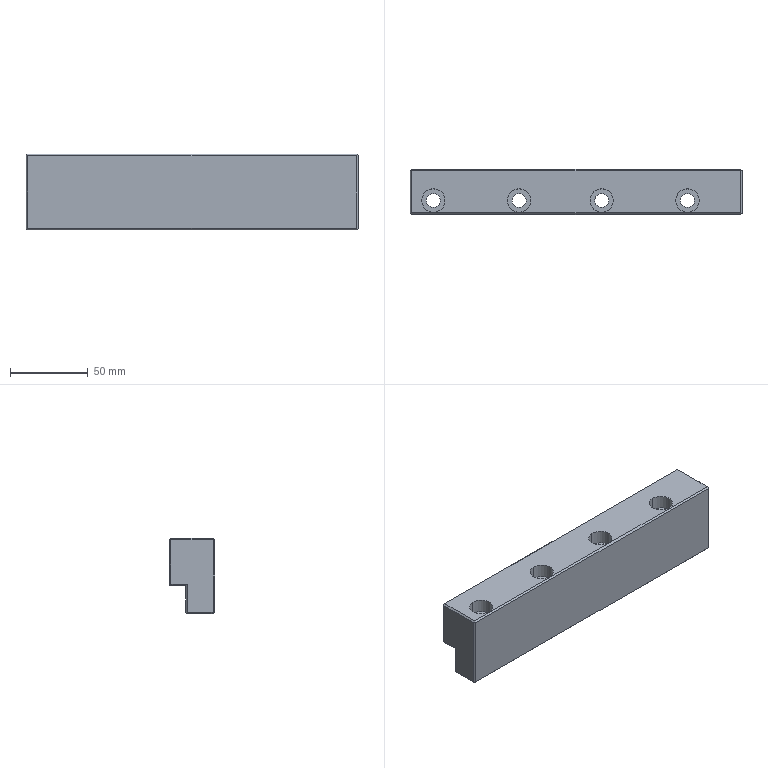Part | Creo | 1 solid | 45 faces | box 213 x 29 x 48.5 mm | volume 242313 mm3 | plane 29 | cylinder 16 | commonest cylinder face diameters 9 x8 15 x8
STEP:
#1=CARTESIAN_POINT('',(333.,-175.005,-11.991));
#2=VERTEX_POINT('',#1);
#3=CARTESIAN_POINT('',(333.,-175.005,-40.991));
#4=VERTEX_POINT('',#3);
#5=CARTESIAN_POINT('',(333.,-175.005,-11.991));
#6=DIRECTION('',(0.,0.,-1.));
#7=VECTOR('',#6,29.);
#8=LINE('',#5,#7);
#9=EDGE_CURVE('',#2,#4,#8,.T.);
#10=ORIENTED_EDGE('',*,*,#9,.F.);
#11=CARTESIAN_POINT('',(122.,-175.005,-11.991));
#12=VERTEX_POINT('',#11);
#13=CARTESIAN_POINT('',(333.,-175.005,-11.991));
#14=DIRECTION('',(-1.,0.,0.));
#15=VECTOR('',#14,211.);
#16=LINE('',#13,#15);
#17=EDGE_CURVE('',#2,#12,#16,.T.);
#18=ORIENTED_EDGE('',*,*,#17,.T.);
#19=CARTESIAN_POINT('',(122.,-175.005,-40.991));
#20=VERTEX_POINT('',#19);
#21=CARTESIAN_POINT('',(122.,-175.005,-40.991));
#22=DIRECTION('',(0.,0.,1.));
#23=VECTOR('',#22,29.);
#24=LINE('',#21,#23);
#25=EDGE_CURVE('',#20,#12,#24,.T.);
#26=ORIENTED_EDGE('',*,*,#25,.F.);
#27=CARTESIAN_POINT('',(333.,-175.005,-40.991));
#28=DIRECTION('',(-1.,0.,0.));
#29=VECTOR('',#28,211.);
#30=LINE('',#27,#29);
#31=EDGE_CURVE('',#4,#20,#30,.T.);
#32=ORIENTED_EDGE('',*,*,#31,.F.);
#33=EDGE_LOOP('',(#10,#18,#26,#32));
#34=FACE_OUTER_BOUND('',#33,.F.);
#35=CARTESIAN_POINT('',(284.,-175.005,3.509));
#36=DIRECTION('',(0.,1.,0.));
#37=DIRECTION('',(0.,0.,-1.));
#38=AXIS2_PLACEMENT_3D('',#35,#36,#37);
#39=PLANE('',#38);
#40=ADVANCED_FACE('',(#34),#39,.T.);
#41=CARTESIAN_POINT('',(334.,-176.005,-11.991));
#42=VERTEX_POINT('',#41);
#43=CARTESIAN_POINT('',(333.5,-175.505,-11.491));
#44=VERTEX_POINT('',#43);
#45=CARTESIAN_POINT('',(334.,-176.005,-11.991));
#46=DIRECTION('',(-0.5774,0.5774,0.5774));
#47=VECTOR('',#46,0.866);
#48=LINE('',#45,#47);
#49=EDGE_CURVE('',#42,#44,#48,.T.);
#50=ORIENTED_EDGE('',*,*,#49,.T.);
#51=CARTESIAN_POINT('',(333.5,-175.505,-11.491));
#52=DIRECTION('',(-0.5774,0.5774,-0.5774));
#53=VECTOR('',#52,0.866);
#54=LINE('',#51,#53);
#55=EDGE_CURVE('',#44,#2,#54,.T.);
#56=ORIENTED_EDGE('',*,*,#55,.T.);
#57=ORIENTED_EDGE('',*,*,#9,.T.);
#58=CARTESIAN_POINT('',(333.25,-175.255,-41.241));
#59=VERTEX_POINT('',#58);
#60=CARTESIAN_POINT('',(333.,-175.005,-40.991));
#61=DIRECTION('',(0.5774,-0.5774,-0.5774));
#62=VECTOR('',#61,0.433);
#63=LINE('',#60,#62);
#64=EDGE_CURVE('',#4,#59,#63,.T.);
#65=ORIENTED_EDGE('',*,*,#64,.T.);
#66=CARTESIAN_POINT('',(334.,-176.005,-40.491));
#67=VERTEX_POINT('',#66);
#68=CARTESIAN_POINT('',(334.,-176.005,-40.491));
#69=DIRECTION('',(-0.5774,0.5774,-0.5774));
#70=VECTOR('',#69,1.299);
#71=LINE('',#68,#70);
#72=EDGE_CURVE('',#67,#59,#71,.T.);
#73=ORIENTED_EDGE('',*,*,#72,.F.);
#74=CARTESIAN_POINT('',(334.,-176.005,-11.991));
#75=DIRECTION('',(0.,0.,-1.));
#76=VECTOR('',#75,28.5);
#77=LINE('',#74,#76);
#78=EDGE_CURVE('',#42,#67,#77,.T.);
#79=ORIENTED_EDGE('',*,*,#78,.F.);
#80=EDGE_LOOP('',(#50,#56,#57,#65,#73,#79));
#81=FACE_OUTER_BOUND('',#80,.F.);
#82=CARTESIAN_POINT('',(333.5,-175.505,-16.491));
#83=DIRECTION('',(0.7071,0.7071,0.));
#84=DIRECTION('',(-0.7071,0.7071,0.));
#85=AXIS2_PLACEMENT_3D('',#82,#83,#84);
#86=PLANE('',#85);
#87=ADVANCED_FACE('',(#81),#86,.T.);
#88=CARTESIAN_POINT('',(333.,-203.005,-10.991));
#89=VERTEX_POINT('',#88);
#90=CARTESIAN_POINT('',(333.,-176.005,-10.991));
#91=VERTEX_POINT('',#90);
#92=CARTESIAN_POINT('',(333.,-203.005,-10.991));
#93=DIRECTION('',(0.,1.,0.));
#94=VECTOR('',#93,27.);
#95=LINE('',#92,#94);
#96=EDGE_CURVE('',#89,#91,#95,.T.);
#97=ORIENTED_EDGE('',*,*,#96,.T.);
#98=CARTESIAN_POINT('',(333.,-176.005,-10.991));
#99=DIRECTION('',(0.5774,0.5774,-0.5774));
#100=VECTOR('',#99,0.866);
#101=LINE('',#98,#100);
#102=EDGE_CURVE('',#91,#44,#101,.T.);
#103=ORIENTED_EDGE('',*,*,#102,.T.);
#104=ORIENTED_EDGE('',*,*,#49,.F.);
#105=CARTESIAN_POINT('',(334.,-203.005,-11.991));
#106=VERTEX_POINT('',#105);
#107=CARTESIAN_POINT('',(334.,-203.005,-11.991));
#108=DIRECTION('',(0.,1.,0.));
#109=VECTOR('',#108,27.);
#110=LINE('',#107,#109);
#111=EDGE_CURVE('',#106,#42,#110,.T.);
#112=ORIENTED_EDGE('',*,*,#111,.F.);
#113=CARTESIAN_POINT('',(333.5,-203.505,-11.491));
#114=VERTEX_POINT('',#113);
#115=CARTESIAN_POINT('',(334.,-203.005,-11.991));
#116=DIRECTION('',(-0.5774,-0.5774,0.5774));
#117=VECTOR('',#116,0.866);
#118=LINE('',#115,#117);
#119=EDGE_CURVE('',#106,#114,#118,.T.);
#120=ORIENTED_EDGE('',*,*,#119,.T.);
#121=CARTESIAN_POINT('',(333.5,-203.505,-11.491));
#122=DIRECTION('',(-0.5774,0.5774,0.5774));
#123=VECTOR('',#122,0.866);
#124=LINE('',#121,#123);
#125=EDGE_CURVE('',#114,#89,#124,.T.);
#126=ORIENTED_EDGE('',*,*,#125,.T.);
#127=EDGE_LOOP('',(#97,#103,#104,#112,#120,#126));
#128=FACE_OUTER_BOUND('',#127,.F.);
#129=CARTESIAN_POINT('',(333.5,-191.505,-11.491));
#130=DIRECTION('',(0.7071,0.,0.7071));
#131=DIRECTION('',(-0.7071,0.,0.7071));
#132=AXIS2_PLACEMENT_3D('',#129,#130,#131);
#133=PLANE('',#132);
#134=ADVANCED_FACE('',(#128),#133,.T.);
#135=CARTESIAN_POINT('',(122.,-176.005,-10.991));
#136=VERTEX_POINT('',#135);
#137=CARTESIAN_POINT('',(122.,-203.005,-10.991));
#138=VERTEX_POINT('',#137);
#139=CARTESIAN_POINT('',(122.,-176.005,-10.991));
#140=DIRECTION('',(0.,-1.,0.));
#141=VECTOR('',#140,27.);
#142=LINE('',#139,#141);
#143=EDGE_CURVE('',#136,#138,#142,.T.);
#144=ORIENTED_EDGE('',*,*,#143,.F.);
#145=CARTESIAN_POINT('',(333.,-176.005,-10.991));
#146=DIRECTION('',(-1.,0.,0.));
#147=VECTOR('',#146,211.);
#148=LINE('',#145,#147);
#149=EDGE_CURVE('',#91,#136,#148,.T.);
#150=ORIENTED_EDGE('',*,*,#149,.F.);
#151=ORIENTED_EDGE('',*,*,#96,.F.);
#152=CARTESIAN_POINT('',(333.,-203.005,-10.991));
#153=DIRECTION('',(-1.,0.,0.));
#154=VECTOR('',#153,211.);
#155=LINE('',#152,#154);
#156=EDGE_CURVE('',#89,#138,#155,.T.);
#157=ORIENTED_EDGE('',*,*,#156,.T.);
#158=EDGE_LOOP('',(#144,#150,#151,#157));
#159=FACE_OUTER_BOUND('',#158,.F.);
#160=CARTESIAN_POINT('',(244.,-202.505,-10.991));
#161=VERTEX_POINT('',#160);
#162=CARTESIAN_POINT('',(244.,-187.505,-10.991));
#163=VERTEX_POINT('',#162);
#164=CARTESIAN_POINT('',(244.,-195.005,-10.991));
#165=DIRECTION('',(0.,0.,-1.));
#166=DIRECTION('',(0.,-1.,0.));
#167=AXIS2_PLACEMENT_3D('',#164,#165,#166);
#168=CIRCLE('',#167,7.5);
#169=EDGE_CURVE('',#161,#163,#168,.T.);
#170=ORIENTED_EDGE('',*,*,#169,.F.);
#171=CARTESIAN_POINT('',(244.,-195.005,-10.991));
#172=DIRECTION('',(0.,0.,-1.));
#173=DIRECTION('',(0.,1.,0.));
#174=AXIS2_PLACEMENT_3D('',#171,#172,#173);
#175=CIRCLE('',#174,7.5);
#176=EDGE_CURVE('',#163,#161,#175,.T.);
#177=ORIENTED_EDGE('',*,*,#176,.F.);
#178=EDGE_LOOP('',(#170,#177));
#179=FACE_BOUND('',#178,.F.);
#180=CARTESIAN_POINT('',(299.,-202.505,-10.991));
#181=VERTEX_POINT('',#180);
#182=CARTESIAN_POINT('',(299.,-187.505,-10.991));
#183=VERTEX_POINT('',#182);
#184=CARTESIAN_POINT('',(299.,-195.005,-10.991));
#185=DIRECTION('',(0.,0.,-1.));
#186=DIRECTION('',(0.,-1.,0.));
#187=AXIS2_PLACEMENT_3D('',#184,#185,#186);
#188=CIRCLE('',#187,7.5);
#189=EDGE_CURVE('',#181,#183,#188,.T.);
#190=ORIENTED_EDGE('',*,*,#189,.F.);
#191=CARTESIAN_POINT('',(299.,-195.005,-10.991));
#192=DIRECTION('',(0.,0.,-1.));
#193=DIRECTION('',(0.,1.,0.));
#194=AXIS2_PLACEMENT_3D('',#191,#192,#193);
#195=CIRCLE('',#194,7.5);
#196=EDGE_CURVE('',#183,#181,#195,.T.);
#197=ORIENTED_EDGE('',*,*,#196,.F.);
#198=EDGE_LOOP('',(#190,#197));
#199=FACE_BOUND('',#198,.F.);
#200=CARTESIAN_POINT('',(136.,-202.505,-10.991));
#201=VERTEX_POINT('',#200);
#202=CARTESIAN_POINT('',(136.,-187.505,-10.991));
#203=VERTEX_POINT('',#202);
#204=CARTESIAN_POINT('',(136.,-195.005,-10.991));
#205=DIRECTION('',(0.,0.,-1.));
#206=DIRECTION('',(0.,-1.,0.));
#207=AXIS2_PLACEMENT_3D('',#204,#205,#206);
#208=CIRCLE('',#207,7.5);
#209=EDGE_CURVE('',#201,#203,#208,.T.);
#210=ORIENTED_EDGE('',*,*,#209,.F.);
#211=CARTESIAN_POINT('',(136.,-195.005,-10.991));
#212=DIRECTION('',(0.,0.,-1.));
#213=DIRECTION('',(0.,1.,0.));
#214=AXIS2_PLACEMENT_3D('',#211,#212,#213);
#215=CIRCLE('',#214,7.5);
#216=EDGE_CURVE('',#203,#201,#215,.T.);
#217=ORIENTED_EDGE('',*,*,#216,.F.);
#218=EDGE_LOOP('',(#210,#217));
#219=FACE_BOUND('',#218,.F.);
#220=CARTESIAN_POINT('',(191.,-202.505,-10.991));
#221=VERTEX_POINT('',#220);
#222=CARTESIAN_POINT('',(191.,-187.505,-10.991));
#223=VERTEX_POINT('',#222);
#224=CARTESIAN_POINT('',(191.,-195.005,-10.991));
#225=DIRECTION('',(0.,0.,-1.));
#226=DIRECTION('',(0.,-1.,0.));
#227=AXIS2_PLACEMENT_3D('',#224,#225,#226);
#228=CIRCLE('',#227,7.5);
#229=EDGE_CURVE('',#221,#223,#228,.T.);
#230=ORIENTED_EDGE('',*,*,#229,.F.);
#231=CARTESIAN_POINT('',(191.,-195.005,-10.991));
#232=DIRECTION('',(0.,0.,-1.));
#233=DIRECTION('',(0.,1.,0.));
#234=AXIS2_PLACEMENT_3D('',#231,#232,#233);
#235=CIRCLE('',#234,7.5);
#236=EDGE_CURVE('',#223,#221,#235,.T.);
#237=ORIENTED_EDGE('',*,*,#236,.F.);
#238=EDGE_LOOP('',(#230,#237));
#239=FACE_BOUND('',#238,.F.);
#240=CARTESIAN_POINT('',(284.,-204.005,-10.991));
#241=DIRECTION('',(0.,0.,1.));
#242=DIRECTION('',(0.,1.,0.));
#243=AXIS2_PLACEMENT_3D('',#240,#241,#242);
#244=PLANE('',#243);
#245=ADVANCED_FACE('',(#159,#179,#199,#219,#239),#244,.T.);
#246=CARTESIAN_POINT('',(191.,-187.505,-19.991));
#247=VERTEX_POINT('',#246);
#248=CARTESIAN_POINT('',(191.,-202.505,-19.991));
#249=VERTEX_POINT('',#248);
#250=CARTESIAN_POINT('',(191.,-195.005,-19.991));
#251=DIRECTION('',(0.,0.,1.));
#252=DIRECTION('',(0.,1.,0.));
#253=AXIS2_PLACEMENT_3D('',#250,#251,#252);
#254=CIRCLE('',#253,7.5);
#255=EDGE_CURVE('',#247,#249,#254,.T.);
#256=ORIENTED_EDGE('',*,*,#255,.T.);
#257=CARTESIAN_POINT('',(191.,-202.505,-10.991));
#258=DIRECTION('',(0.,0.,-1.));
#259=VECTOR('',#258,9.);
#260=LINE('',#257,#259);
#261=EDGE_CURVE('',#221,#249,#260,.T.);
#262=ORIENTED_EDGE('',*,*,#261,.F.);
#263=ORIENTED_EDGE('',*,*,#229,.T.);
#264=CARTESIAN_POINT('',(191.,-187.505,-10.991));
#265=DIRECTION('',(0.,0.,-1.));
#266=VECTOR('',#265,9.);
#267=LINE('',#264,#266);
#268=EDGE_CURVE('',#223,#247,#267,.T.);
#269=ORIENTED_EDGE('',*,*,#268,.T.);
#270=EDGE_LOOP('',(#256,#262,#263,#269));
#271=FACE_OUTER_BOUND('',#270,.F.);
#272=CARTESIAN_POINT('',(191.,-195.005,-10.541));
#273=DIRECTION('',(0.,0.,-1.));
#274=DIRECTION('',(0.,-1.,0.));
#275=AXIS2_PLACEMENT_3D('',#272,#273,#274);
#276=CYLINDRICAL_SURFACE('',#275,7.5);
#277=ADVANCED_FACE('',(#271),#276,.F.);
#278=CARTESIAN_POINT('',(191.,-195.005,-19.991));
#279=DIRECTION('',(0.,0.,1.));
#280=DIRECTION('',(0.,-1.,0.));
#281=AXIS2_PLACEMENT_3D('',#278,#279,#280);
#282=CIRCLE('',#281,7.5);
#283=EDGE_CURVE('',#249,#247,#282,.T.);
#284=ORIENTED_EDGE('',*,*,#283,.F.);
#285=ORIENTED_EDGE('',*,*,#255,.F.);
#286=EDGE_LOOP('',(#284,#285));
#287=FACE_OUTER_BOUND('',#286,.F.);
#288=CARTESIAN_POINT('',(191.,-199.505,-19.991));
#289=VERTEX_POINT('',#288);
#290=CARTESIAN_POINT('',(191.,-190.505,-19.991));
#291=VERTEX_POINT('',#290);
#292=CARTESIAN_POINT('',(191.,-195.005,-19.991));
#293=DIRECTION('',(0.,0.,-1.));
#294=DIRECTION('',(0.,-1.,0.));
#295=AXIS2_PLACEMENT_3D('',#292,#293,#294);
#296=CIRCLE('',#295,4.5);
#297=EDGE_CURVE('',#289,#291,#296,.T.);
#298=ORIENTED_EDGE('',*,*,#297,.F.);
#299=CARTESIAN_POINT('',(191.,-195.005,-19.991));
#300=DIRECTION('',(0.,0.,-1.));
#301=DIRECTION('',(0.,1.,0.));
#302=AXIS2_PLACEMENT_3D('',#299,#300,#301);
#303=CIRCLE('',#302,4.5);
#304=EDGE_CURVE('',#291,#289,#303,.T.);
#305=ORIENTED_EDGE('',*,*,#304,.F.);
#306=EDGE_LOOP('',(#298,#305));
#307=FACE_BOUND('',#306,.F.);
#308=CARTESIAN_POINT('',(191.,-195.005,-19.991));
#309=DIRECTION('',(0.,0.,-1.));
#310=DIRECTION('',(0.,-1.,0.));
#311=AXIS2_PLACEMENT_3D('',#308,#309,#310);
#312=PLANE('',#311);
#313=ADVANCED_FACE('',(#287,#307),#312,.F.);
#314=CARTESIAN_POINT('',(191.,-190.505,-59.491));
#315=VERTEX_POINT('',#314);
#316=CARTESIAN_POINT('',(191.,-199.505,-59.491));
#317=VERTEX_POINT('',#316);
#318=CARTESIAN_POINT('',(191.,-195.005,-59.491));
#319=DIRECTION('',(0.,0.,1.));
#320=DIRECTION('',(0.,1.,0.));
#321=AXIS2_PLACEMENT_3D('',#318,#319,#320);
#322=CIRCLE('',#321,4.5);
#323=EDGE_CURVE('',#315,#317,#322,.T.);
#324=ORIENTED_EDGE('',*,*,#323,.T.);
#325=CARTESIAN_POINT('',(191.,-199.505,-59.491));
#326=DIRECTION('',(0.,0.,1.));
#327=VECTOR('',#326,39.5);
#328=LINE('',#325,#327);
#329=EDGE_CURVE('',#317,#289,#328,.T.);
#330=ORIENTED_EDGE('',*,*,#329,.T.);
#331=ORIENTED_EDGE('',*,*,#297,.T.);
#332=CARTESIAN_POINT('',(191.,-190.505,-59.491));
#333=DIRECTION('',(0.,0.,1.));
#334=VECTOR('',#333,39.5);
#335=LINE('',#332,#334);
#336=EDGE_CURVE('',#315,#291,#335,.T.);
#337=ORIENTED_EDGE('',*,*,#336,.F.);
#338=EDGE_LOOP('',(#324,#330,#331,#337));
#339=FACE_OUTER_BOUND('',#338,.F.);
#340=CARTESIAN_POINT('',(191.,-195.005,-5.491));
#341=DIRECTION('',(0.,0.,1.));
#342=DIRECTION('',(0.,-1.,0.));
#343=AXIS2_PLACEMENT_3D('',#340,#341,#342);
#344=CYLINDRICAL_SURFACE('',#343,4.5);
#345=ADVANCED_FACE('',(#339),#344,.F.);
#346=CARTESIAN_POINT('',(333.,-186.505,-59.491));
#347=VERTEX_POINT('',#346);
#348=CARTESIAN_POINT('',(333.,-203.005,-59.491));
#349=VERTEX_POINT('',#348);
#350=CARTESIAN_POINT('',(333.,-186.505,-59.491));
#351=DIRECTION('',(0.,-1.,0.));
#352=VECTOR('',#351,16.5);
#353=LINE('',#350,#352);
#354=EDGE_CURVE('',#347,#349,#353,.T.);
#355=ORIENTED_EDGE('',*,*,#354,.F.);
#356=CARTESIAN_POINT('',(122.,-186.505,-59.491));
#357=VERTEX_POINT('',#356);
#358=CARTESIAN_POINT('',(333.,-186.505,-59.491));
#359=DIRECTION('',(-1.,0.,0.));
#360=VECTOR('',#359,211.);
#361=LINE('',#358,#360);
#362=EDGE_CURVE('',#347,#357,#361,.T.);
#363=ORIENTED_EDGE('',*,*,#362,.T.);
#364=CARTESIAN_POINT('',(122.,-203.005,-59.491));
#365=VERTEX_POINT('',#364);
#366=CARTESIAN_POINT('',(122.,-203.005,-59.491));
#367=DIRECTION('',(0.,1.,0.));
#368=VECTOR('',#367,16.5);
#369=LINE('',#366,#368);
#370=EDGE_CURVE('',#365,#357,#369,.T.);
#371=ORIENTED_EDGE('',*,*,#370,.F.);
#372=CARTESIAN_POINT('',(333.,-203.005,-59.491));
#373=DIRECTION('',(-1.,0.,0.));
#374=VECTOR('',#373,211.);
#375=LINE('',#372,#374);
#376=EDGE_CURVE('',#349,#365,#375,.T.);
#377=ORIENTED_EDGE('',*,*,#376,.F.);
#378=EDGE_LOOP('',(#355,#363,#371,#377));
#379=FACE_OUTER_BOUND('',#378,.F.);
#380=CARTESIAN_POINT('',(244.,-199.505,-59.491));
#381=VERTEX_POINT('',#380);
#382=CARTESIAN_POINT('',(244.,-190.505,-59.491));
#383=VERTEX_POINT('',#382);
#384=CARTESIAN_POINT('',(244.,-195.005,-59.491));
#385=DIRECTION('',(0.,0.,1.));
#386=DIRECTION('',(0.,-1.,0.));
#387=AXIS2_PLACEMENT_3D('',#384,#385,#386);
#388=CIRCLE('',#387,4.5);
#389=EDGE_CURVE('',#381,#383,#388,.T.);
#390=ORIENTED_EDGE('',*,*,#389,.F.);
#391=CARTESIAN_POINT('',(244.,-195.005,-59.491));
#392=DIRECTION('',(0.,0.,1.));
#393=DIRECTION('',(0.,1.,0.));
#394=AXIS2_PLACEMENT_3D('',#391,#392,#393);
#395=CIRCLE('',#394,4.5);
#396=EDGE_CURVE('',#383,#381,#395,.T.);
#397=ORIENTED_EDGE('',*,*,#396,.F.);
#398=EDGE_LOOP('',(#390,#397));
#399=FACE_BOUND('',#398,.F.);
#400=CARTESIAN_POINT('',(299.,-199.505,-59.491));
#401=VERTEX_POINT('',#400);
#402=CARTESIAN_POINT('',(299.,-190.505,-59.491));
#403=VERTEX_POINT('',#402);
#404=CARTESIAN_POINT('',(299.,-195.005,-59.491));
#405=DIRECTION('',(0.,0.,1.));
#406=DIRECTION('',(0.,-1.,0.));
#407=AXIS2_PLACEMENT_3D('',#404,#405,#406);
#408=CIRCLE('',#407,4.5);
#409=EDGE_CURVE('',#401,#403,#408,.T.);
#410=ORIENTED_EDGE('',*,*,#409,.F.);
#411=CARTESIAN_POINT('',(299.,-195.005,-59.491));
#412=DIRECTION('',(0.,0.,1.));
#413=DIRECTION('',(0.,1.,0.));
#414=AXIS2_PLACEMENT_3D('',#411,#412,#413);
#415=CIRCLE('',#414,4.5);
#416=EDGE_CURVE('',#403,#401,#415,.T.);
#417=ORIENTED_EDGE('',*,*,#416,.F.);
#418=EDGE_LOOP('',(#410,#417));
#419=FACE_BOUND('',#418,.F.);
#420=CARTESIAN_POINT('',(136.,-199.505,-59.491));
#421=VERTEX_POINT('',#420);
#422=CARTESIAN_POINT('',(136.,-190.505,-59.491));
#423=VERTEX_POINT('',#422);
#424=CARTESIAN_POINT('',(136.,-195.005,-59.491));
#425=DIRECTION('',(0.,0.,1.));
#426=DIRECTION('',(0.,-1.,0.));
#427=AXIS2_PLACEMENT_3D('',#424,#425,#426);
#428=CIRCLE('',#427,4.5);
#429=EDGE_CURVE('',#421,#423,#428,.T.);
#430=ORIENTED_EDGE('',*,*,#429,.F.);
#431=CARTESIAN_POINT('',(136.,-195.005,-59.491));
#432=DIRECTION('',(0.,0.,1.));
#433=DIRECTION('',(0.,1.,0.));
#434=AXIS2_PLACEMENT_3D('',#431,#432,#433);
#435=CIRCLE('',#434,4.5);
#436=EDGE_CURVE('',#423,#421,#435,.T.);
#437=ORIENTED_EDGE('',*,*,#436,.F.);
#438=EDGE_LOOP('',(#430,#437));
#439=FACE_BOUND('',#438,.F.);
#440=CARTESIAN_POINT('',(191.,-195.005,-59.491));
#441=DIRECTION('',(0.,0.,1.));
#442=DIRECTION('',(0.,-1.,0.));
#443=AXIS2_PLACEMENT_3D('',#440,#441,#442);
#444=CIRCLE('',#443,4.5);
#445=EDGE_CURVE('',#317,#315,#444,.T.);
#446=ORIENTED_EDGE('',*,*,#445,.F.);
#447=ORIENTED_EDGE('',*,*,#323,.F.);
#448=EDGE_LOOP('',(#446,#447));
#449=FACE_BOUND('',#448,.F.);
#450=CARTESIAN_POINT('',(284.,-185.505,-59.491));
#451=DIRECTION('',(0.,0.,-1.));
#452=DIRECTION('',(0.,-1.,0.));
#453=AXIS2_PLACEMENT_3D('',#450,#451,#452);
#454=PLANE('',#453);
#455=ADVANCED_FACE('',(#379,#399,#419,#439,#449),#454,.T.);
#456=ORIENTED_EDGE('',*,*,#445,.T.);
#457=ORIENTED_EDGE('',*,*,#336,.T.);
#458=ORIENTED_EDGE('',*,*,#304,.T.);
#459=ORIENTED_EDGE('',*,*,#329,.F.);
#460=EDGE_LOOP('',(#456,#457,#458,#459));
#461=FACE_OUTER_BOUND('',#460,.F.);
#462=CARTESIAN_POINT('',(191.,-195.005,-5.491));
#463=DIRECTION('',(0.,0.,1.));
#464=DIRECTION('',(0.,-1.,0.));
#465=AXIS2_PLACEMENT_3D('',#462,#463,#464);
#466=CYLINDRICAL_SURFACE('',#465,4.5);
#467=ADVANCED_FACE('',(#461),#466,.F.);
#468=ORIENTED_EDGE('',*,*,#389,.T.);
#469=CARTESIAN_POINT('',(244.,-190.505,-19.991));
#470=VERTEX_POINT('',#469);
#471=CARTESIAN_POINT('',(244.,-190.505,-59.491));
#472=DIRECTION('',(0.,0.,1.));
#473=VECTOR('',#472,39.5);
#474=LINE('',#471,#473);
#475=EDGE_CURVE('',#383,#470,#474,.T.);
#476=ORIENTED_EDGE('',*,*,#475,.T.);
#477=CARTESIAN_POINT('',(244.,-199.505,-19.991));
#478=VERTEX_POINT('',#477);
#479=CARTESIAN_POINT('',(244.,-195.005,-19.991));
#480=DIRECTION('',(0.,0.,-1.));
#481=DIRECTION('',(0.,1.,0.));
#482=AXIS2_PLACEMENT_3D('',#479,#480,#481);
#483=CIRCLE('',#482,4.5);
#484=EDGE_CURVE('',#470,#478,#483,.T.);
#485=ORIENTED_EDGE('',*,*,#484,.T.);
#486=CARTESIAN_POINT('',(244.,-199.505,-59.491));
#487=DIRECTION('',(0.,0.,1.));
#488=VECTOR('',#487,39.5);
#489=LINE('',#486,#488);
#490=EDGE_CURVE('',#381,#478,#489,.T.);
#491=ORIENTED_EDGE('',*,*,#490,.F.);
#492=EDGE_LOOP('',(#468,#476,#485,#491));
#493=FACE_OUTER_BOUND('',#492,.F.);
#494=CARTESIAN_POINT('',(244.,-195.005,-5.491));
#495=DIRECTION('',(0.,0.,1.));
#496=DIRECTION('',(0.,-1.,0.));
#497=AXIS2_PLACEMENT_3D('',#494,#495,#496);
#498=CYLINDRICAL_SURFACE('',#497,4.5);
#499=ADVANCED_FACE('',(#493),#498,.F.);
#500=ORIENTED_EDGE('',*,*,#396,.T.);
#501=ORIENTED_EDGE('',*,*,#490,.T.);
#502=CARTESIAN_POINT('',(244.,-195.005,-19.991));
#503=DIRECTION('',(0.,0.,-1.));
#504=DIRECTION('',(0.,-1.,0.));
#505=AXIS2_PLACEMENT_3D('',#502,#503,#504);
#506=CIRCLE('',#505,4.5);
#507=EDGE_CURVE('',#478,#470,#506,.T.);
#508=ORIENTED_EDGE('',*,*,#507,.T.);
#509=ORIENTED_EDGE('',*,*,#475,.F.);
#510=EDGE_LOOP('',(#500,#501,#508,#509));
#511=FACE_OUTER_BOUND('',#510,.F.);
#512=CARTESIAN_POINT('',(244.,-195.005,-5.491));
#513=DIRECTION('',(0.,0.,1.));
#514=DIRECTION('',(0.,-1.,0.));
#515=AXIS2_PLACEMENT_3D('',#512,#513,#514);
#516=CYLINDRICAL_SURFACE('',#515,4.5);
#517=ADVANCED_FACE('',(#511),#516,.F.);
#518=CARTESIAN_POINT('',(244.,-202.505,-19.991));
#519=VERTEX_POINT('',#518);
#520=CARTESIAN_POINT('',(244.,-187.505,-19.991));
#521=VERTEX_POINT('',#520);
#522=CARTESIAN_POINT('',(244.,-195.005,-19.991));
#523=DIRECTION('',(0.,0.,1.));
#524=DIRECTION('',(0.,-1.,0.));
#525=AXIS2_PLACEMENT_3D('',#522,#523,#524);
#526=CIRCLE('',#525,7.5);
#527=EDGE_CURVE('',#519,#521,#526,.T.);
#528=ORIENTED_EDGE('',*,*,#527,.F.);
#529=CARTESIAN_POINT('',(244.,-195.005,-19.991));
#530=DIRECTION('',(0.,0.,1.));
#531=DIRECTION('',(0.,1.,0.));
#532=AXIS2_PLACEMENT_3D('',#529,#530,#531);
#533=CIRCLE('',#532,7.5);
#534=EDGE_CURVE('',#521,#519,#533,.T.);
#535=ORIENTED_EDGE('',*,*,#534,.F.);
#536=EDGE_LOOP('',(#528,#535));
#537=FACE_OUTER_BOUND('',#536,.F.);
#538=ORIENTED_EDGE('',*,*,#507,.F.);
#539=ORIENTED_EDGE('',*,*,#484,.F.);
#540=EDGE_LOOP('',(#538,#539));
#541=FACE_BOUND('',#540,.F.);
#542=CARTESIAN_POINT('',(244.,-195.005,-19.991));
#543=DIRECTION('',(0.,0.,-1.));
#544=DIRECTION('',(0.,-1.,0.));
#545=AXIS2_PLACEMENT_3D('',#542,#543,#544);
#546=PLANE('',#545);
#547=ADVANCED_FACE('',(#537,#541),#546,.F.);
#548=ORIENTED_EDGE('',*,*,#527,.T.);
#549=CARTESIAN_POINT('',(244.,-187.505,-10.991));
#550=DIRECTION('',(0.,0.,-1.));
#551=VECTOR('',#550,9.);
#552=LINE('',#549,#551);
#553=EDGE_CURVE('',#163,#521,#552,.T.);
#554=ORIENTED_EDGE('',*,*,#553,.F.);
#555=ORIENTED_EDGE('',*,*,#176,.T.);
#556=CARTESIAN_POINT('',(244.,-202.505,-10.991));
#557=DIRECTION('',(0.,0.,-1.));
#558=VECTOR('',#557,9.);
#559=LINE('',#556,#558);
#560=EDGE_CURVE('',#161,#519,#559,.T.);
#561=ORIENTED_EDGE('',*,*,#560,.T.);
#562=EDGE_LOOP('',(#548,#554,#555,#561));
#563=FACE_OUTER_BOUND('',#562,.F.);
#564=CARTESIAN_POINT('',(244.,-195.005,-10.541));
#565=DIRECTION('',(0.,0.,-1.));
#566=DIRECTION('',(0.,-1.,0.));
#567=AXIS2_PLACEMENT_3D('',#564,#565,#566);
#568=CYLINDRICAL_SURFACE('',#567,7.5);
#569=ADVANCED_FACE('',(#563),#568,.F.);
#570=ORIENTED_EDGE('',*,*,#534,.T.);
#571=ORIENTED_EDGE('',*,*,#560,.F.);
#572=ORIENTED_EDGE('',*,*,#169,.T.);
#573=ORIENTED_EDGE('',*,*,#553,.T.);
#574=EDGE_LOOP('',(#570,#571,#572,#573));
#575=FACE_OUTER_BOUND('',#574,.F.);
#576=CARTESIAN_POINT('',(244.,-195.005,-10.541));
#577=DIRECTION('',(0.,0.,-1.));
#578=DIRECTION('',(0.,-1.,0.));
#579=AXIS2_PLACEMENT_3D('',#576,#577,#578);
#580=CYLINDRICAL_SURFACE('',#579,7.5);
#581=ADVANCED_FACE('',(#575),#580,.F.);
#582=ORIENTED_EDGE('',*,*,#409,.T.);
#583=CARTESIAN_POINT('',(299.,-190.505,-19.991));
#584=VERTEX_POINT('',#583);
#585=CARTESIAN_POINT('',(299.,-190.505,-59.491));
#586=DIRECTION('',(0.,0.,1.));
#587=VECTOR('',#586,39.5);
#588=LINE('',#585,#587);
#589=EDGE_CURVE('',#403,#584,#588,.T.);
#590=ORIENTED_EDGE('',*,*,#589,.T.);
#591=CARTESIAN_POINT('',(299.,-199.505,-19.991));
#592=VERTEX_POINT('',#591);
#593=CARTESIAN_POINT('',(299.,-195.005,-19.991));
#594=DIRECTION('',(0.,0.,-1.));
#595=DIRECTION('',(0.,1.,0.));
#596=AXIS2_PLACEMENT_3D('',#593,#594,#595);
#597=CIRCLE('',#596,4.5);
#598=EDGE_CURVE('',#584,#592,#597,.T.);
#599=ORIENTED_EDGE('',*,*,#598,.T.);
#600=CARTESIAN_POINT('',(299.,-199.505,-59.491));
#601=DIRECTION('',(0.,0.,1.));
#602=VECTOR('',#601,39.5);
#603=LINE('',#600,#602);
#604=EDGE_CURVE('',#401,#592,#603,.T.);
#605=ORIENTED_EDGE('',*,*,#604,.F.);
#606=EDGE_LOOP('',(#582,#590,#599,#605));
#607=FACE_OUTER_BOUND('',#606,.F.);
#608=CARTESIAN_POINT('',(299.,-195.005,-5.491));
#609=DIRECTION('',(0.,0.,1.));
#610=DIRECTION('',(0.,-1.,0.));
#611=AXIS2_PLACEMENT_3D('',#608,#609,#610);
#612=CYLINDRICAL_SURFACE('',#611,4.5);
#613=ADVANCED_FACE('',(#607),#612,.F.);
#614=ORIENTED_EDGE('',*,*,#416,.T.);
#615=ORIENTED_EDGE('',*,*,#604,.T.);
#616=CARTESIAN_POINT('',(299.,-195.005,-19.991));
#617=DIRECTION('',(0.,0.,-1.));
#618=DIRECTION('',(0.,-1.,0.));
#619=AXIS2_PLACEMENT_3D('',#616,#617,#618);
#620=CIRCLE('',#619,4.5);
#621=EDGE_CURVE('',#592,#584,#620,.T.);
#622=ORIENTED_EDGE('',*,*,#621,.T.);
#623=ORIENTED_EDGE('',*,*,#589,.F.);
#624=EDGE_LOOP('',(#614,#615,#622,#623));
#625=FACE_OUTER_BOUND('',#624,.F.);
#626=CARTESIAN_POINT('',(299.,-195.005,-5.491));
#627=DIRECTION('',(0.,0.,1.));
#628=DIRECTION('',(0.,-1.,0.));
#629=AXIS2_PLACEMENT_3D('',#626,#627,#628);
#630=CYLINDRICAL_SURFACE('',#629,4.5);
#631=ADVANCED_FACE('',(#625),#630,.F.);
#632=CARTESIAN_POINT('',(299.,-202.505,-19.991));
#633=VERTEX_POINT('',#632);
#634=CARTESIAN_POINT('',(299.,-187.505,-19.991));
#635=VERTEX_POINT('',#634);
#636=CARTESIAN_POINT('',(299.,-195.005,-19.991));
#637=DIRECTION('',(0.,0.,1.));
#638=DIRECTION('',(0.,-1.,0.));
#639=AXIS2_PLACEMENT_3D('',#636,#637,#638);
#640=CIRCLE('',#639,7.5);
#641=EDGE_CURVE('',#633,#635,#640,.T.);
#642=ORIENTED_EDGE('',*,*,#641,.F.);
#643=CARTESIAN_POINT('',(299.,-195.005,-19.991));
#644=DIRECTION('',(0.,0.,1.));
#645=DIRECTION('',(0.,1.,0.));
#646=AXIS2_PLACEMENT_3D('',#643,#644,#645);
#647=CIRCLE('',#646,7.5);
#648=EDGE_CURVE('',#635,#633,#647,.T.);
#649=ORIENTED_EDGE('',*,*,#648,.F.);
#650=EDGE_LOOP('',(#642,#649));
#651=FACE_OUTER_BOUND('',#650,.F.);
#652=ORIENTED_EDGE('',*,*,#621,.F.);
#653=ORIENTED_EDGE('',*,*,#598,.F.);
#654=EDGE_LOOP('',(#652,#653));
#655=FACE_BOUND('',#654,.F.);
#656=CARTESIAN_POINT('',(299.,-195.005,-19.991));
#657=DIRECTION('',(0.,0.,-1.));
#658=DIRECTION('',(0.,-1.,0.));
#659=AXIS2_PLACEMENT_3D('',#656,#657,#658);
#660=PLANE('',#659);
#661=ADVANCED_FACE('',(#651,#655),#660,.F.);
#662=ORIENTED_EDGE('',*,*,#641,.T.);
#663=CARTESIAN_POINT('',(299.,-187.505,-10.991));
#664=DIRECTION('',(0.,0.,-1.));
#665=VECTOR('',#664,9.);
#666=LINE('',#663,#665);
#667=EDGE_CURVE('',#183,#635,#666,.T.);
#668=ORIENTED_EDGE('',*,*,#667,.F.);
#669=ORIENTED_EDGE('',*,*,#196,.T.);
#670=CARTESIAN_POINT('',(299.,-202.505,-10.991));
#671=DIRECTION('',(0.,0.,-1.));
#672=VECTOR('',#671,9.);
#673=LINE('',#670,#672);
#674=EDGE_CURVE('',#181,#633,#673,.T.);
#675=ORIENTED_EDGE('',*,*,#674,.T.);
#676=EDGE_LOOP('',(#662,#668,#669,#675));
#677=FACE_OUTER_BOUND('',#676,.F.);
#678=CARTESIAN_POINT('',(299.,-195.005,-10.541));
#679=DIRECTION('',(0.,0.,-1.));
#680=DIRECTION('',(0.,-1.,0.));
#681=AXIS2_PLACEMENT_3D('',#678,#679,#680);
#682=CYLINDRICAL_SURFACE('',#681,7.5);
#683=ADVANCED_FACE('',(#677),#682,.F.);
#684=ORIENTED_EDGE('',*,*,#648,.T.);
#685=ORIENTED_EDGE('',*,*,#674,.F.);
#686=ORIENTED_EDGE('',*,*,#189,.T.);
#687=ORIENTED_EDGE('',*,*,#667,.T.);
#688=EDGE_LOOP('',(#684,#685,#686,#687));
#689=FACE_OUTER_BOUND('',#688,.F.);
#690=CARTESIAN_POINT('',(299.,-195.005,-10.541));
#691=DIRECTION('',(0.,0.,-1.));
#692=DIRECTION('',(0.,-1.,0.));
#693=AXIS2_PLACEMENT_3D('',#690,#691,#692);
#694=CYLINDRICAL_SURFACE('',#693,7.5);
#695=ADVANCED_FACE('',(#689),#694,.F.);
#696=ORIENTED_EDGE('',*,*,#429,.T.);
#697=CARTESIAN_POINT('',(136.,-190.505,-19.991));
#698=VERTEX_POINT('',#697);
#699=CARTESIAN_POINT('',(136.,-190.505,-59.491));
#700=DIRECTION('',(0.,0.,1.));
#701=VECTOR('',#700,39.5);
#702=LINE('',#699,#701);
#703=EDGE_CURVE('',#423,#698,#702,.T.);
#704=ORIENTED_EDGE('',*,*,#703,.T.);
#705=CARTESIAN_POINT('',(136.,-199.505,-19.991));
#706=VERTEX_POINT('',#705);
#707=CARTESIAN_POINT('',(136.,-195.005,-19.991));
#708=DIRECTION('',(0.,0.,-1.));
#709=DIRECTION('',(0.,1.,0.));
#710=AXIS2_PLACEMENT_3D('',#707,#708,#709);
#711=CIRCLE('',#710,4.5);
#712=EDGE_CURVE('',#698,#706,#711,.T.);
#713=ORIENTED_EDGE('',*,*,#712,.T.);
#714=CARTESIAN_POINT('',(136.,-199.505,-59.491));
#715=DIRECTION('',(0.,0.,1.));
#716=VECTOR('',#715,39.5);
#717=LINE('',#714,#716);
#718=EDGE_CURVE('',#421,#706,#717,.T.);
#719=ORIENTED_EDGE('',*,*,#718,.F.);
#720=EDGE_LOOP('',(#696,#704,#713,#719));
#721=FACE_OUTER_BOUND('',#720,.F.);
#722=CARTESIAN_POINT('',(136.,-195.005,-5.491));
#723=DIRECTION('',(0.,0.,1.));
#724=DIRECTION('',(0.,-1.,0.));
#725=AXIS2_PLACEMENT_3D('',#722,#723,#724);
#726=CYLINDRICAL_SURFACE('',#725,4.5);
#727=ADVANCED_FACE('',(#721),#726,.F.);
#728=ORIENTED_EDGE('',*,*,#436,.T.);
#729=ORIENTED_EDGE('',*,*,#718,.T.);
#730=CARTESIAN_POINT('',(136.,-195.005,-19.991));
#731=DIRECTION('',(0.,0.,-1.));
#732=DIRECTION('',(0.,-1.,0.));
#733=AXIS2_PLACEMENT_3D('',#730,#731,#732);
#734=CIRCLE('',#733,4.5);
#735=EDGE_CURVE('',#706,#698,#734,.T.);
#736=ORIENTED_EDGE('',*,*,#735,.T.);
#737=ORIENTED_EDGE('',*,*,#703,.F.);
#738=EDGE_LOOP('',(#728,#729,#736,#737));
#739=FACE_OUTER_BOUND('',#738,.F.);
#740=CARTESIAN_POINT('',(136.,-195.005,-5.491));
#741=DIRECTION('',(0.,0.,1.));
#742=DIRECTION('',(0.,-1.,0.));
#743=AXIS2_PLACEMENT_3D('',#740,#741,#742);
#744=CYLINDRICAL_SURFACE('',#743,4.5);
#745=ADVANCED_FACE('',(#739),#744,.F.);
#746=CARTESIAN_POINT('',(136.,-202.505,-19.991));
#747=VERTEX_POINT('',#746);
#748=CARTESIAN_POINT('',(136.,-187.505,-19.991));
#749=VERTEX_POINT('',#748);
#750=CARTESIAN_POINT('',(136.,-195.005,-19.991));
#751=DIRECTION('',(0.,0.,1.));
#752=DIRECTION('',(0.,-1.,0.));
#753=AXIS2_PLACEMENT_3D('',#750,#751,#752);
#754=CIRCLE('',#753,7.5);
#755=EDGE_CURVE('',#747,#749,#754,.T.);
#756=ORIENTED_EDGE('',*,*,#755,.F.);
#757=CARTESIAN_POINT('',(136.,-195.005,-19.991));
#758=DIRECTION('',(0.,0.,1.));
#759=DIRECTION('',(0.,1.,0.));
#760=AXIS2_PLACEMENT_3D('',#757,#758,#759);
#761=CIRCLE('',#760,7.5);
#762=EDGE_CURVE('',#749,#747,#761,.T.);
#763=ORIENTED_EDGE('',*,*,#762,.F.);
#764=EDGE_LOOP('',(#756,#763));
#765=FACE_OUTER_BOUND('',#764,.F.);
#766=ORIENTED_EDGE('',*,*,#735,.F.);
#767=ORIENTED_EDGE('',*,*,#712,.F.);
#768=EDGE_LOOP('',(#766,#767));
#769=FACE_BOUND('',#768,.F.);
#770=CARTESIAN_POINT('',(136.,-195.005,-19.991));
#771=DIRECTION('',(0.,0.,-1.));
#772=DIRECTION('',(0.,-1.,0.));
#773=AXIS2_PLACEMENT_3D('',#770,#771,#772);
#774=PLANE('',#773);
#775=ADVANCED_FACE('',(#765,#769),#774,.F.);
#776=ORIENTED_EDGE('',*,*,#755,.T.);
#777=CARTESIAN_POINT('',(136.,-187.505,-10.991));
#778=DIRECTION('',(0.,0.,-1.));
#779=VECTOR('',#778,9.);
#780=LINE('',#777,#779);
#781=EDGE_CURVE('',#203,#749,#780,.T.);
#782=ORIENTED_EDGE('',*,*,#781,.F.);
#783=ORIENTED_EDGE('',*,*,#216,.T.);
#784=CARTESIAN_POINT('',(136.,-202.505,-10.991));
#785=DIRECTION('',(0.,0.,-1.));
#786=VECTOR('',#785,9.);
#787=LINE('',#784,#786);
#788=EDGE_CURVE('',#201,#747,#787,.T.);
#789=ORIENTED_EDGE('',*,*,#788,.T.);
#790=EDGE_LOOP('',(#776,#782,#783,#789));
#791=FACE_OUTER_BOUND('',#790,.F.);
#792=CARTESIAN_POINT('',(136.,-195.005,-10.541));
#793=DIRECTION('',(0.,0.,-1.));
#794=DIRECTION('',(0.,-1.,0.));
#795=AXIS2_PLACEMENT_3D('',#792,#793,#794);
#796=CYLINDRICAL_SURFACE('',#795,7.5);
#797=ADVANCED_FACE('',(#791),#796,.F.);
#798=ORIENTED_EDGE('',*,*,#762,.T.);
#799=ORIENTED_EDGE('',*,*,#788,.F.);
#800=ORIENTED_EDGE('',*,*,#209,.T.);
#801=ORIENTED_EDGE('',*,*,#781,.T.);
#802=EDGE_LOOP('',(#798,#799,#800,#801));
#803=FACE_OUTER_BOUND('',#802,.F.);
#804=CARTESIAN_POINT('',(136.,-195.005,-10.541));
#805=DIRECTION('',(0.,0.,-1.));
#806=DIRECTION('',(0.,-1.,0.));
#807=AXIS2_PLACEMENT_3D('',#804,#805,#806);
#808=CYLINDRICAL_SURFACE('',#807,7.5);
#809=ADVANCED_FACE('',(#803),#808,.F.);
#810=CARTESIAN_POINT('',(333.5,-186.005,-58.991));
#811=VERTEX_POINT('',#810);
#812=CARTESIAN_POINT('',(333.5,-186.005,-58.991));
#813=DIRECTION('',(-0.5774,-0.5774,-0.5774));
#814=VECTOR('',#813,0.866);
#815=LINE('',#812,#814);
#816=EDGE_CURVE('',#811,#347,#815,.T.);
#817=ORIENTED_EDGE('',*,*,#816,.T.);
#818=ORIENTED_EDGE('',*,*,#354,.T.);
#819=CARTESIAN_POINT('',(333.5,-203.505,-58.991));
#820=VERTEX_POINT('',#819);
#821=CARTESIAN_POINT('',(333.5,-203.505,-58.991));
#822=DIRECTION('',(-0.5774,0.5774,-0.5774));
#823=VECTOR('',#822,0.866);
#824=LINE('',#821,#823);
#825=EDGE_CURVE('',#820,#349,#824,.T.);
#826=ORIENTED_EDGE('',*,*,#825,.F.);
#827=CARTESIAN_POINT('',(334.,-203.005,-58.491));
#828=VERTEX_POINT('',#827);
#829=CARTESIAN_POINT('',(333.5,-203.505,-58.991));
#830=DIRECTION('',(0.5774,0.5774,0.5774));
#831=VECTOR('',#830,0.866);
#832=LINE('',#829,#831);
#833=EDGE_CURVE('',#820,#828,#832,.T.);
#834=ORIENTED_EDGE('',*,*,#833,.T.);
#835=CARTESIAN_POINT('',(334.,-186.505,-58.491));
#836=VERTEX_POINT('',#835);
#837=CARTESIAN_POINT('',(334.,-186.505,-58.491));
#838=DIRECTION('',(0.,-1.,0.));
#839=VECTOR('',#838,16.5);
#840=LINE('',#837,#839);
#841=EDGE_CURVE('',#836,#828,#840,.T.);
#842=ORIENTED_EDGE('',*,*,#841,.F.);
#843=CARTESIAN_POINT('',(334.,-186.505,-58.491));
#844=DIRECTION('',(-0.5774,0.5774,-0.5774));
#845=VECTOR('',#844,0.866);
#846=LINE('',#843,#845);
#847=EDGE_CURVE('',#836,#811,#846,.T.);
#848=ORIENTED_EDGE('',*,*,#847,.T.);
#849=EDGE_LOOP('',(#817,#818,#826,#834,#842,#848));
#850=FACE_OUTER_BOUND('',#849,.F.);
#851=CARTESIAN_POINT('',(333.5,-194.755,-58.991));
#852=DIRECTION('',(0.7071,0.,-0.7071));
#853=DIRECTION('',(-0.7071,0.,-0.7071));
#854=AXIS2_PLACEMENT_3D('',#851,#852,#853);
#855=PLANE('',#854);
#856=ADVANCED_FACE('',(#850),#855,.T.);
#857=CARTESIAN_POINT('',(121.5,-186.005,-58.991));
#858=VERTEX_POINT('',#857);
#859=CARTESIAN_POINT('',(121.5,-186.005,-58.991));
#860=DIRECTION('',(0.5774,-0.5774,-0.5774));
#861=VECTOR('',#860,0.866);
#862=LINE('',#859,#861);
#863=EDGE_CURVE('',#858,#357,#862,.T.);
#864=ORIENTED_EDGE('',*,*,#863,.T.);
#865=ORIENTED_EDGE('',*,*,#362,.F.);
#866=ORIENTED_EDGE('',*,*,#816,.F.);
#867=CARTESIAN_POINT('',(333.,-185.505,-58.491));
#868=VERTEX_POINT('',#867);
#869=CARTESIAN_POINT('',(333.5,-186.005,-58.991));
#870=DIRECTION('',(-0.5774,0.5774,0.5774));
#871=VECTOR('',#870,0.866);
#872=LINE('',#869,#871);
#873=EDGE_CURVE('',#811,#868,#872,.T.);
#874=ORIENTED_EDGE('',*,*,#873,.T.);
#875=CARTESIAN_POINT('',(122.,-185.505,-58.491));
#876=VERTEX_POINT('',#875);
#877=CARTESIAN_POINT('',(333.,-185.505,-58.491));
#878=DIRECTION('',(-1.,0.,0.));
#879=VECTOR('',#878,211.);
#880=LINE('',#877,#879);
#881=EDGE_CURVE('',#868,#876,#880,.T.);
#882=ORIENTED_EDGE('',*,*,#881,.T.);
#883=CARTESIAN_POINT('',(122.,-185.505,-58.491));
#884=DIRECTION('',(-0.5774,-0.5774,-0.5774));
#885=VECTOR('',#884,0.866);
#886=LINE('',#883,#885);
#887=EDGE_CURVE('',#876,#858,#886,.T.);
#888=ORIENTED_EDGE('',*,*,#887,.T.);
#889=EDGE_LOOP('',(#864,#865,#866,#874,#882,#888));
#890=FACE_OUTER_BOUND('',#889,.F.);
#891=CARTESIAN_POINT('',(202.5,-186.005,-58.991));
#892=DIRECTION('',(0.,0.7071,-0.7071));
#893=DIRECTION('',(0.,0.7071,0.7071));
#894=AXIS2_PLACEMENT_3D('',#891,#892,#893);
#895=PLANE('',#894);
#896=ADVANCED_FACE('',(#890),#895,.T.);
#897=CARTESIAN_POINT('',(121.,-186.505,-58.491));
#898=VERTEX_POINT('',#897);
#899=CARTESIAN_POINT('',(121.5,-186.005,-58.991));
#900=DIRECTION('',(-0.5774,-0.5774,0.5774));
#901=VECTOR('',#900,0.866);
#902=LINE('',#899,#901);
#903=EDGE_CURVE('',#858,#898,#902,.T.);
#904=ORIENTED_EDGE('',*,*,#903,.T.);
#905=CARTESIAN_POINT('',(121.,-203.005,-58.491));
#906=VERTEX_POINT('',#905);
#907=CARTESIAN_POINT('',(121.,-203.005,-58.491));
#908=DIRECTION('',(0.,1.,0.));
#909=VECTOR('',#908,16.5);
#910=LINE('',#907,#909);
#911=EDGE_CURVE('',#906,#898,#910,.T.);
#912=ORIENTED_EDGE('',*,*,#911,.F.);
#913=CARTESIAN_POINT('',(121.5,-203.505,-58.991));
#914=VERTEX_POINT('',#913);
#915=CARTESIAN_POINT('',(121.,-203.005,-58.491));
#916=DIRECTION('',(0.5774,-0.5774,-0.5774));
#917=VECTOR('',#916,0.866);
#918=LINE('',#915,#917);
#919=EDGE_CURVE('',#906,#914,#918,.T.);
#920=ORIENTED_EDGE('',*,*,#919,.T.);
#921=CARTESIAN_POINT('',(121.5,-203.505,-58.991));
#922=DIRECTION('',(0.5774,0.5774,-0.5774));
#923=VECTOR('',#922,0.866);
#924=LINE('',#921,#923);
#925=EDGE_CURVE('',#914,#365,#924,.T.);
#926=ORIENTED_EDGE('',*,*,#925,.T.);
#927=ORIENTED_EDGE('',*,*,#370,.T.);
#928=ORIENTED_EDGE('',*,*,#863,.F.);
#929=EDGE_LOOP('',(#904,#912,#920,#926,#927,#928));
#930=FACE_OUTER_BOUND('',#929,.F.);
#931=CARTESIAN_POINT('',(121.5,-194.755,-58.991));
#932=DIRECTION('',(-0.7071,0.,-0.7071));
#933=DIRECTION('',(0.7071,0.,-0.7071));
#934=AXIS2_PLACEMENT_3D('',#931,#932,#933);
#935=PLANE('',#934);
#936=ADVANCED_FACE('',(#930),#935,.T.);
#937=ORIENTED_EDGE('',*,*,#887,.F.);
#938=CARTESIAN_POINT('',(122.,-185.505,-41.491));
#939=VERTEX_POINT('',#938);
#940=CARTESIAN_POINT('',(122.,-185.505,-58.491));
#941=DIRECTION('',(0.,0.,1.));
#942=VECTOR('',#941,17.);
#943=LINE('',#940,#942);
#944=EDGE_CURVE('',#876,#939,#943,.T.);
#945=ORIENTED_EDGE('',*,*,#944,.T.);
#946=CARTESIAN_POINT('',(121.,-186.505,-40.491));
#947=VERTEX_POINT('',#946);
#948=CARTESIAN_POINT('',(121.,-186.505,-40.491));
#949=DIRECTION('',(0.5774,0.5774,-0.5774));
#950=VECTOR('',#949,1.732);
#951=LINE('',#948,#950);
#952=EDGE_CURVE('',#947,#939,#951,.T.);
#953=ORIENTED_EDGE('',*,*,#952,.F.);
#954=CARTESIAN_POINT('',(121.,-186.505,-58.491));
#955=DIRECTION('',(0.,0.,1.));
#956=VECTOR('',#955,18.);
#957=LINE('',#954,#956);
#958=EDGE_CURVE('',#898,#947,#957,.T.);
#959=ORIENTED_EDGE('',*,*,#958,.F.);
#960=ORIENTED_EDGE('',*,*,#903,.F.);
#961=EDGE_LOOP('',(#937,#945,#953,#959,#960));
#962=FACE_OUTER_BOUND('',#961,.F.);
#963=CARTESIAN_POINT('',(121.5,-186.005,-44.491));
#964=DIRECTION('',(-0.7071,0.7071,0.));
#965=DIRECTION('',(0.7071,0.7071,0.));
#966=AXIS2_PLACEMENT_3D('',#963,#964,#965);
#967=PLANE('',#966);
#968=ADVANCED_FACE('',(#962),#967,.T.);
#969=CARTESIAN_POINT('',(333.,-185.505,-41.491));
#970=VERTEX_POINT('',#969);
#971=CARTESIAN_POINT('',(122.,-185.505,-41.491));
#972=DIRECTION('',(1.,0.,0.));
#973=VECTOR('',#972,211.);
#974=LINE('',#971,#973);
#975=EDGE_CURVE('',#939,#970,#974,.T.);
#976=ORIENTED_EDGE('',*,*,#975,.F.);
#977=ORIENTED_EDGE('',*,*,#944,.F.);
#978=ORIENTED_EDGE('',*,*,#881,.F.);
#979=CARTESIAN_POINT('',(333.,-185.505,-41.491));
#980=DIRECTION('',(0.,0.,-1.));
#981=VECTOR('',#980,17.);
#982=LINE('',#979,#981);
#983=EDGE_CURVE('',#970,#868,#982,.T.);
#984=ORIENTED_EDGE('',*,*,#983,.F.);
#985=EDGE_LOOP('',(#976,#977,#978,#984));
#986=FACE_OUTER_BOUND('',#985,.F.);
#987=CARTESIAN_POINT('',(284.,-185.505,-36.491));
#988=DIRECTION('',(0.,1.,0.));
#989=DIRECTION('',(0.,0.,-1.));
#990=AXIS2_PLACEMENT_3D('',#987,#988,#989);
#991=PLANE('',#990);
#992=ADVANCED_FACE('',(#986),#991,.T.);
#993=CARTESIAN_POINT('',(333.,-175.505,-41.491));
#994=VERTEX_POINT('',#993);
#995=CARTESIAN_POINT('',(333.,-175.505,-41.491));
#996=DIRECTION('',(0.,-1.,0.));
#997=VECTOR('',#996,10.);
#998=LINE('',#995,#997);
#999=EDGE_CURVE('',#994,#970,#998,.T.);
#1000=ORIENTED_EDGE('',*,*,#999,.F.);
#1001=CARTESIAN_POINT('',(122.,-175.505,-41.491));
#1002=VERTEX_POINT('',#1001);
#1003=CARTESIAN_POINT('',(333.,-175.505,-41.491));
#1004=DIRECTION('',(-1.,0.,0.));
#1005=VECTOR('',#1004,211.);
#1006=LINE('',#1003,#1005);
#1007=EDGE_CURVE('',#994,#1002,#1006,.T.);
#1008=ORIENTED_EDGE('',*,*,#1007,.T.);
#1009=CARTESIAN_POINT('',(122.,-185.505,-41.491));
#1010=DIRECTION('',(0.,1.,0.));
#1011=VECTOR('',#1010,10.);
#1012=LINE('',#1009,#1011);
#1013=EDGE_CURVE('',#939,#1002,#1012,.T.);
#1014=ORIENTED_EDGE('',*,*,#1013,.F.);
#1015=ORIENTED_EDGE('',*,*,#975,.T.);
#1016=EDGE_LOOP('',(#1000,#1008,#1014,#1015));
#1017=FACE_OUTER_BOUND('',#1016,.F.);
#1018=CARTESIAN_POINT('',(284.,-179.005,-41.491));
#1019=DIRECTION('',(0.,0.,-1.));
#1020=DIRECTION('',(0.,-1.,0.));
#1021=AXIS2_PLACEMENT_3D('',#1018,#1019,#1020);
#1022=PLANE('',#1021);
#1023=ADVANCED_FACE('',(#1017),#1022,.T.);
#1024=ORIENTED_EDGE('',*,*,#72,.T.);
#1025=CARTESIAN_POINT('',(333.25,-175.255,-41.241));
#1026=DIRECTION('',(-0.5774,-0.5774,-0.5774));
#1027=VECTOR('',#1026,0.433);
#1028=LINE('',#1025,#1027);
#1029=EDGE_CURVE('',#59,#994,#1028,.T.);
#1030=ORIENTED_EDGE('',*,*,#1029,.T.);
#1031=ORIENTED_EDGE('',*,*,#999,.T.);
#1032=CARTESIAN_POINT('',(334.,-186.505,-40.491));
#1033=VERTEX_POINT('',#1032);
#1034=CARTESIAN_POINT('',(334.,-186.505,-40.491));
#1035=DIRECTION('',(-0.5774,0.5774,-0.5774));
#1036=VECTOR('',#1035,1.732);
#1037=LINE('',#1034,#1036);
#1038=EDGE_CURVE('',#1033,#970,#1037,.T.);
#1039=ORIENTED_EDGE('',*,*,#1038,.F.);
#1040=CARTESIAN_POINT('',(334.,-176.005,-40.491));
#1041=DIRECTION('',(0.,-1.,0.));
#1042=VECTOR('',#1041,10.5);
#1043=LINE('',#1040,#1042);
#1044=EDGE_CURVE('',#67,#1033,#1043,.T.);
#1045=ORIENTED_EDGE('',*,*,#1044,.F.);
#1046=EDGE_LOOP('',(#1024,#1030,#1031,#1039,#1045));
#1047=FACE_OUTER_BOUND('',#1046,.F.);
#1048=CARTESIAN_POINT('',(333.5,-182.255,-40.991));
#1049=DIRECTION('',(0.7071,0.,-0.7071));
#1050=DIRECTION('',(-0.7071,0.,-0.7071));
#1051=AXIS2_PLACEMENT_3D('',#1048,#1049,#1050);
#1052=PLANE('',#1051);
#1053=ADVANCED_FACE('',(#1047),#1052,.T.);
#1054=ORIENTED_EDGE('',*,*,#1007,.F.);
#1055=ORIENTED_EDGE('',*,*,#1029,.F.);
#1056=ORIENTED_EDGE('',*,*,#64,.F.);
#1057=ORIENTED_EDGE('',*,*,#31,.T.);
#1058=CARTESIAN_POINT('',(121.75,-175.255,-41.241));
#1059=VERTEX_POINT('',#1058);
#1060=CARTESIAN_POINT('',(121.75,-175.255,-41.241));
#1061=DIRECTION('',(0.5774,0.5774,0.5774));
#1062=VECTOR('',#1061,0.433);
#1063=LINE('',#1060,#1062);
#1064=EDGE_CURVE('',#1059,#20,#1063,.T.);
#1065=ORIENTED_EDGE('',*,*,#1064,.F.);
#1066=CARTESIAN_POINT('',(122.,-175.505,-41.491));
#1067=DIRECTION('',(-0.5774,0.5774,0.5774));
#1068=VECTOR('',#1067,0.433);
#1069=LINE('',#1066,#1068);
#1070=EDGE_CURVE('',#1002,#1059,#1069,.T.);
#1071=ORIENTED_EDGE('',*,*,#1070,.F.);
#1072=EDGE_LOOP('',(#1054,#1055,#1056,#1057,#1065,#1071));
#1073=FACE_OUTER_BOUND('',#1072,.F.);
#1074=CARTESIAN_POINT('',(202.5,-175.255,-41.241));
#1075=DIRECTION('',(0.,0.7071,-0.7071));
#1076=DIRECTION('',(0.,0.7071,0.7071));
#1077=AXIS2_PLACEMENT_3D('',#1074,#1075,#1076);
#1078=PLANE('',#1077);
#1079=ADVANCED_FACE('',(#1073),#1078,.T.);
#1080=ORIENTED_EDGE('',*,*,#25,.T.);
#1081=CARTESIAN_POINT('',(121.5,-175.505,-11.491));
#1082=VERTEX_POINT('',#1081);
#1083=CARTESIAN_POINT('',(122.,-175.005,-11.991));
#1084=DIRECTION('',(-0.5774,-0.5774,0.5774));
#1085=VECTOR('',#1084,0.866);
#1086=LINE('',#1083,#1085);
#1087=EDGE_CURVE('',#12,#1082,#1086,.T.);
#1088=ORIENTED_EDGE('',*,*,#1087,.T.);
#1089=CARTESIAN_POINT('',(121.,-176.005,-11.991));
#1090=VERTEX_POINT('',#1089);
#1091=CARTESIAN_POINT('',(121.,-176.005,-11.991));
#1092=DIRECTION('',(0.5774,0.5774,0.5774));
#1093=VECTOR('',#1092,0.866);
#1094=LINE('',#1091,#1093);
#1095=EDGE_CURVE('',#1090,#1082,#1094,.T.);
#1096=ORIENTED_EDGE('',*,*,#1095,.F.);
#1097=CARTESIAN_POINT('',(121.,-176.005,-40.491));
#1098=VERTEX_POINT('',#1097);
#1099=CARTESIAN_POINT('',(121.,-176.005,-40.491));
#1100=DIRECTION('',(0.,0.,1.));
#1101=VECTOR('',#1100,28.5);
#1102=LINE('',#1099,#1101);
#1103=EDGE_CURVE('',#1098,#1090,#1102,.T.);
#1104=ORIENTED_EDGE('',*,*,#1103,.F.);
#1105=CARTESIAN_POINT('',(121.,-176.005,-40.491));
#1106=DIRECTION('',(0.5774,0.5774,-0.5774));
#1107=VECTOR('',#1106,1.299);
#1108=LINE('',#1105,#1107);
#1109=EDGE_CURVE('',#1098,#1059,#1108,.T.);
#1110=ORIENTED_EDGE('',*,*,#1109,.T.);
#1111=ORIENTED_EDGE('',*,*,#1064,.T.);
#1112=EDGE_LOOP('',(#1080,#1088,#1096,#1104,#1110,#1111));
#1113=FACE_OUTER_BOUND('',#1112,.F.);
#1114=CARTESIAN_POINT('',(121.5,-175.505,-16.491));
#1115=DIRECTION('',(-0.7071,0.7071,0.));
#1116=DIRECTION('',(0.7071,0.7071,0.));
#1117=AXIS2_PLACEMENT_3D('',#1114,#1115,#1116);
#1118=PLANE('',#1117);
#1119=ADVANCED_FACE('',(#1113),#1118,.T.);
#1120=ORIENTED_EDGE('',*,*,#17,.F.);
#1121=ORIENTED_EDGE('',*,*,#55,.F.);
#1122=ORIENTED_EDGE('',*,*,#102,.F.);
#1123=ORIENTED_EDGE('',*,*,#149,.T.);
#1124=CARTESIAN_POINT('',(121.5,-175.505,-11.491));
#1125=DIRECTION('',(0.5774,-0.5774,0.5774));
#1126=VECTOR('',#1125,0.866);
#1127=LINE('',#1124,#1126);
#1128=EDGE_CURVE('',#1082,#136,#1127,.T.);
#1129=ORIENTED_EDGE('',*,*,#1128,.F.);
#1130=ORIENTED_EDGE('',*,*,#1087,.F.);
#1131=EDGE_LOOP('',(#1120,#1121,#1122,#1123,#1129,#1130));
#1132=FACE_OUTER_BOUND('',#1131,.F.);
#1133=CARTESIAN_POINT('',(202.5,-175.505,-11.491));
#1134=DIRECTION('',(0.,0.7071,0.7071));
#1135=DIRECTION('',(0.,-0.7071,0.7071));
#1136=AXIS2_PLACEMENT_3D('',#1133,#1134,#1135);
#1137=PLANE('',#1136);
#1138=ADVANCED_FACE('',(#1132),#1137,.T.);
#1139=ORIENTED_EDGE('',*,*,#1095,.T.);
#1140=ORIENTED_EDGE('',*,*,#1128,.T.);
#1141=ORIENTED_EDGE('',*,*,#143,.T.);
#1142=CARTESIAN_POINT('',(121.5,-203.505,-11.491));
#1143=VERTEX_POINT('',#1142);
#1144=CARTESIAN_POINT('',(121.5,-203.505,-11.491));
#1145=DIRECTION('',(0.5774,0.5774,0.5774));
#1146=VECTOR('',#1145,0.866);
#1147=LINE('',#1144,#1146);
#1148=EDGE_CURVE('',#1143,#138,#1147,.T.);
#1149=ORIENTED_EDGE('',*,*,#1148,.F.);
#1150=CARTESIAN_POINT('',(121.,-203.005,-11.991));
#1151=VERTEX_POINT('',#1150);
#1152=CARTESIAN_POINT('',(121.5,-203.505,-11.491));
#1153=DIRECTION('',(-0.5774,0.5774,-0.5774));
#1154=VECTOR('',#1153,0.866);
#1155=LINE('',#1152,#1154);
#1156=EDGE_CURVE('',#1143,#1151,#1155,.T.);
#1157=ORIENTED_EDGE('',*,*,#1156,.T.);
#1158=CARTESIAN_POINT('',(121.,-176.005,-11.991));
#1159=DIRECTION('',(0.,-1.,0.));
#1160=VECTOR('',#1159,27.);
#1161=LINE('',#1158,#1160);
#1162=EDGE_CURVE('',#1090,#1151,#1161,.T.);
#1163=ORIENTED_EDGE('',*,*,#1162,.F.);
#1164=EDGE_LOOP('',(#1139,#1140,#1141,#1149,#1157,#1163));
#1165=FACE_OUTER_BOUND('',#1164,.F.);
#1166=CARTESIAN_POINT('',(121.5,-191.505,-11.491));
#1167=DIRECTION('',(-0.7071,0.,0.7071));
#1168=DIRECTION('',(0.7071,0.,0.7071));
#1169=AXIS2_PLACEMENT_3D('',#1166,#1167,#1168);
#1170=PLANE('',#1169);
#1171=ADVANCED_FACE('',(#1165),#1170,.T.);
#1172=ORIENTED_EDGE('',*,*,#1148,.T.);
#1173=ORIENTED_EDGE('',*,*,#156,.F.);
#1174=ORIENTED_EDGE('',*,*,#125,.F.);
#1175=CARTESIAN_POINT('',(333.,-204.005,-11.991));
#1176=VERTEX_POINT('',#1175);
#1177=CARTESIAN_POINT('',(333.5,-203.505,-11.491));
#1178=DIRECTION('',(-0.5774,-0.5774,-0.5774));
#1179=VECTOR('',#1178,0.866);
#1180=LINE('',#1177,#1179);
#1181=EDGE_CURVE('',#114,#1176,#1180,.T.);
#1182=ORIENTED_EDGE('',*,*,#1181,.T.);
#1183=CARTESIAN_POINT('',(122.,-204.005,-11.991));
#1184=VERTEX_POINT('',#1183);
#1185=CARTESIAN_POINT('',(333.,-204.005,-11.991));
#1186=DIRECTION('',(-1.,0.,0.));
#1187=VECTOR('',#1186,211.);
#1188=LINE('',#1185,#1187);
#1189=EDGE_CURVE('',#1176,#1184,#1188,.T.);
#1190=ORIENTED_EDGE('',*,*,#1189,.T.);
#1191=CARTESIAN_POINT('',(122.,-204.005,-11.991));
#1192=DIRECTION('',(-0.5774,0.5774,0.5774));
#1193=VECTOR('',#1192,0.866);
#1194=LINE('',#1191,#1193);
#1195=EDGE_CURVE('',#1184,#1143,#1194,.T.);
#1196=ORIENTED_EDGE('',*,*,#1195,.T.);
#1197=EDGE_LOOP('',(#1172,#1173,#1174,#1182,#1190,#1196));
#1198=FACE_OUTER_BOUND('',#1197,.F.);
#1199=CARTESIAN_POINT('',(202.5,-203.505,-11.491));
#1200=DIRECTION('',(0.,-0.7071,0.7071));
#1201=DIRECTION('',(0.,-0.7071,-0.7071));
#1202=AXIS2_PLACEMENT_3D('',#1199,#1200,#1201);
#1203=PLANE('',#1202);
#1204=ADVANCED_FACE('',(#1198),#1203,.T.);
#1205=CARTESIAN_POINT('',(333.,-204.005,-58.491));
#1206=VERTEX_POINT('',#1205);
#1207=CARTESIAN_POINT('',(333.,-204.005,-58.491));
#1208=DIRECTION('',(0.5774,0.5774,-0.5774));
#1209=VECTOR('',#1208,0.866);
#1210=LINE('',#1207,#1209);
#1211=EDGE_CURVE('',#1206,#820,#1210,.T.);
#1212=ORIENTED_EDGE('',*,*,#1211,.F.);
#1213=CARTESIAN_POINT('',(333.,-204.005,-58.491));
#1214=DIRECTION('',(0.,0.,1.));
#1215=VECTOR('',#1214,46.5);
#1216=LINE('',#1213,#1215);
#1217=EDGE_CURVE('',#1206,#1176,#1216,.T.);
#1218=ORIENTED_EDGE('',*,*,#1217,.T.);
#1219=ORIENTED_EDGE('',*,*,#1181,.F.);
#1220=ORIENTED_EDGE('',*,*,#119,.F.);
#1221=CARTESIAN_POINT('',(334.,-203.005,-58.491));
#1222=DIRECTION('',(0.,0.,1.));
#1223=VECTOR('',#1222,46.5);
#1224=LINE('',#1221,#1223);
#1225=EDGE_CURVE('',#828,#106,#1224,.T.);
#1226=ORIENTED_EDGE('',*,*,#1225,.F.);
#1227=ORIENTED_EDGE('',*,*,#833,.F.);
#1228=EDGE_LOOP('',(#1212,#1218,#1219,#1220,#1226,#1227));
#1229=FACE_OUTER_BOUND('',#1228,.F.);
#1230=CARTESIAN_POINT('',(333.5,-203.505,-24.491));
#1231=DIRECTION('',(0.7071,-0.7071,0.));
#1232=DIRECTION('',(-0.7071,-0.7071,0.));
#1233=AXIS2_PLACEMENT_3D('',#1230,#1231,#1232);
#1234=PLANE('',#1233);
#1235=ADVANCED_FACE('',(#1229),#1234,.T.);
#1236=CARTESIAN_POINT('',(122.,-204.005,-58.491));
#1237=VERTEX_POINT('',#1236);
#1238=CARTESIAN_POINT('',(121.5,-203.505,-58.991));
#1239=DIRECTION('',(0.5774,-0.5774,0.5774));
#1240=VECTOR('',#1239,0.866);
#1241=LINE('',#1238,#1240);
#1242=EDGE_CURVE('',#914,#1237,#1241,.T.);
#1243=ORIENTED_EDGE('',*,*,#1242,.T.);
#1244=CARTESIAN_POINT('',(333.,-204.005,-58.491));
#1245=DIRECTION('',(-1.,0.,0.));
#1246=VECTOR('',#1245,211.);
#1247=LINE('',#1244,#1246);
#1248=EDGE_CURVE('',#1206,#1237,#1247,.T.);
#1249=ORIENTED_EDGE('',*,*,#1248,.F.);
#1250=ORIENTED_EDGE('',*,*,#1211,.T.);
#1251=ORIENTED_EDGE('',*,*,#825,.T.);
#1252=ORIENTED_EDGE('',*,*,#376,.T.);
#1253=ORIENTED_EDGE('',*,*,#925,.F.);
#1254=EDGE_LOOP('',(#1243,#1249,#1250,#1251,#1252,#1253));
#1255=FACE_OUTER_BOUND('',#1254,.F.);
#1256=CARTESIAN_POINT('',(202.5,-203.505,-58.991));
#1257=DIRECTION('',(0.,-0.7071,-0.7071));
#1258=DIRECTION('',(0.,0.7071,-0.7071));
#1259=AXIS2_PLACEMENT_3D('',#1256,#1257,#1258);
#1260=PLANE('',#1259);
#1261=ADVANCED_FACE('',(#1255),#1260,.T.);
#1262=ORIENTED_EDGE('',*,*,#1195,.F.);
#1263=CARTESIAN_POINT('',(122.,-204.005,-11.991));
#1264=DIRECTION('',(0.,0.,-1.));
#1265=VECTOR('',#1264,46.5);
#1266=LINE('',#1263,#1265);
#1267=EDGE_CURVE('',#1184,#1237,#1266,.T.);
#1268=ORIENTED_EDGE('',*,*,#1267,.T.);
#1269=ORIENTED_EDGE('',*,*,#1242,.F.);
#1270=ORIENTED_EDGE('',*,*,#919,.F.);
#1271=CARTESIAN_POINT('',(121.,-203.005,-11.991));
#1272=DIRECTION('',(0.,0.,-1.));
#1273=VECTOR('',#1272,46.5);
#1274=LINE('',#1271,#1273);
#1275=EDGE_CURVE('',#1151,#906,#1274,.T.);
#1276=ORIENTED_EDGE('',*,*,#1275,.F.);
#1277=ORIENTED_EDGE('',*,*,#1156,.F.);
#1278=EDGE_LOOP('',(#1262,#1268,#1269,#1270,#1276,#1277));
#1279=FACE_OUTER_BOUND('',#1278,.F.);
#1280=CARTESIAN_POINT('',(121.5,-203.505,-24.491));
#1281=DIRECTION('',(-0.7071,-0.7071,0.));
#1282=DIRECTION('',(0.7071,-0.7071,0.));
#1283=AXIS2_PLACEMENT_3D('',#1280,#1281,#1282);
#1284=PLANE('',#1283);
#1285=ADVANCED_FACE('',(#1279),#1284,.T.);
#1286=ORIENTED_EDGE('',*,*,#1248,.T.);
#1287=ORIENTED_EDGE('',*,*,#1267,.F.);
#1288=ORIENTED_EDGE('',*,*,#1189,.F.);
#1289=ORIENTED_EDGE('',*,*,#1217,.F.);
#1290=EDGE_LOOP('',(#1286,#1287,#1288,#1289));
#1291=FACE_OUTER_BOUND('',#1290,.F.);
#1292=CARTESIAN_POINT('',(284.,-204.005,-52.491));
#1293=DIRECTION('',(0.,-1.,0.));
#1294=DIRECTION('',(0.,0.,1.));
#1295=AXIS2_PLACEMENT_3D('',#1292,#1293,#1294);
#1296=PLANE('',#1295);
#1297=ADVANCED_FACE('',(#1291),#1296,.T.);
#1298=ORIENTED_EDGE('',*,*,#1162,.T.);
#1299=ORIENTED_EDGE('',*,*,#1275,.T.);
#1300=ORIENTED_EDGE('',*,*,#911,.T.);
#1301=ORIENTED_EDGE('',*,*,#958,.T.);
#1302=CARTESIAN_POINT('',(121.,-186.505,-40.491));
#1303=DIRECTION('',(0.,1.,0.));
#1304=VECTOR('',#1303,10.5);
#1305=LINE('',#1302,#1304);
#1306=EDGE_CURVE('',#947,#1098,#1305,.T.);
#1307=ORIENTED_EDGE('',*,*,#1306,.T.);
#1308=ORIENTED_EDGE('',*,*,#1103,.T.);
#1309=EDGE_LOOP('',(#1298,#1299,#1300,#1301,#1307,#1308));
#1310=FACE_OUTER_BOUND('',#1309,.F.);
#1311=CARTESIAN_POINT('',(121.,-185.505,-36.491));
#1312=DIRECTION('',(-1.,0.,0.));
#1313=DIRECTION('',(0.,0.,1.));
#1314=AXIS2_PLACEMENT_3D('',#1311,#1312,#1313);
#1315=PLANE('',#1314);
#1316=ADVANCED_FACE('',(#1310),#1315,.T.);
#1317=ORIENTED_EDGE('',*,*,#1013,.T.);
#1318=ORIENTED_EDGE('',*,*,#1070,.T.);
#1319=ORIENTED_EDGE('',*,*,#1109,.F.);
#1320=ORIENTED_EDGE('',*,*,#1306,.F.);
#1321=ORIENTED_EDGE('',*,*,#952,.T.);
#1322=EDGE_LOOP('',(#1317,#1318,#1319,#1320,#1321));
#1323=FACE_OUTER_BOUND('',#1322,.F.);
#1324=CARTESIAN_POINT('',(121.5,-182.255,-40.991));
#1325=DIRECTION('',(-0.7071,0.,-0.7071));
#1326=DIRECTION('',(0.7071,0.,-0.7071));
#1327=AXIS2_PLACEMENT_3D('',#1324,#1325,#1326);
#1328=PLANE('',#1327);
#1329=ADVANCED_FACE('',(#1323),#1328,.T.);
#1330=CARTESIAN_POINT('',(334.,-186.505,-40.491));
#1331=DIRECTION('',(0.,0.,-1.));
#1332=VECTOR('',#1331,18.);
#1333=LINE('',#1330,#1332);
#1334=EDGE_CURVE('',#1033,#836,#1333,.T.);
#1335=ORIENTED_EDGE('',*,*,#1334,.T.);
#1336=ORIENTED_EDGE('',*,*,#841,.T.);
#1337=ORIENTED_EDGE('',*,*,#1225,.T.);
#1338=ORIENTED_EDGE('',*,*,#111,.T.);
#1339=ORIENTED_EDGE('',*,*,#78,.T.);
#1340=ORIENTED_EDGE('',*,*,#1044,.T.);
#1341=EDGE_LOOP('',(#1335,#1336,#1337,#1338,#1339,#1340));
#1342=FACE_OUTER_BOUND('',#1341,.F.);
#1343=CARTESIAN_POINT('',(334.,-185.505,-36.491));
#1344=DIRECTION('',(-1.,0.,0.));
#1345=DIRECTION('',(0.,0.,1.));
#1346=AXIS2_PLACEMENT_3D('',#1343,#1344,#1345);
#1347=PLANE('',#1346);
#1348=ADVANCED_FACE('',(#1342),#1347,.F.);
#1349=ORIENTED_EDGE('',*,*,#847,.F.);
#1350=ORIENTED_EDGE('',*,*,#1334,.F.);
#1351=ORIENTED_EDGE('',*,*,#1038,.T.);
#1352=ORIENTED_EDGE('',*,*,#983,.T.);
#1353=ORIENTED_EDGE('',*,*,#873,.F.);
#1354=EDGE_LOOP('',(#1349,#1350,#1351,#1352,#1353));
#1355=FACE_OUTER_BOUND('',#1354,.F.);
#1356=CARTESIAN_POINT('',(333.5,-186.005,-44.491));
#1357=DIRECTION('',(0.7071,0.7071,0.));
#1358=DIRECTION('',(-0.7071,0.7071,0.));
#1359=AXIS2_PLACEMENT_3D('',#1356,#1357,#1358);
#1360=PLANE('',#1359);
#1361=ADVANCED_FACE('',(#1355),#1360,.T.);
#1362=ORIENTED_EDGE('',*,*,#283,.T.);
#1363=ORIENTED_EDGE('',*,*,#268,.F.);
#1364=ORIENTED_EDGE('',*,*,#236,.T.);
#1365=ORIENTED_EDGE('',*,*,#261,.T.);
#1366=EDGE_LOOP('',(#1362,#1363,#1364,#1365));
#1367=FACE_OUTER_BOUND('',#1366,.F.);
#1368=CARTESIAN_POINT('',(191.,-195.005,-10.541));
#1369=DIRECTION('',(0.,0.,-1.));
#1370=DIRECTION('',(0.,-1.,0.));
#1371=AXIS2_PLACEMENT_3D('',#1368,#1369,#1370);
#1372=CYLINDRICAL_SURFACE('',#1371,7.5);
#1373=ADVANCED_FACE('',(#1367),#1372,.F.);
#1374=CLOSED_SHELL('',(#40,#87,#134,#245,#277,#313,#345,#455,#467,#499,#517,#547,#569,#581,#613,#631,#661,#683,#695,#727,#745,#775,#797,#809,#856,#896,#936,#968,#992,#1023,#1053,#1079,#1119,#1138,#1171,#1204,#1235,#1261,#1285,#1297,#1316,#1329,#1348,#1361,#1373));
#1375=MANIFOLD_SOLID_BREP('',#1374);
#1376=(LENGTH_UNIT()NAMED_UNIT(*)SI_UNIT(.MILLI.,.METRE.));
#1377=UNCERTAINTY_MEASURE_WITH_UNIT(LENGTH_MEASURE(0.02204),#1376,'','');
#1378=(NAMED_UNIT(*)PLANE_ANGLE_UNIT()SI_UNIT($,.RADIAN.));
#1379=PLANE_ANGLE_MEASURE_WITH_UNIT(PLANE_ANGLE_MEASURE(0.01745),#1378);
#1380=(CONVERSION_BASED_UNIT('DEGREE',#1379)NAMED_UNIT(*)PLANE_ANGLE_UNIT());
#1381=(NAMED_UNIT(*)SI_UNIT($,.STERADIAN.)SOLID_ANGLE_UNIT());
#1382=(GEOMETRIC_REPRESENTATION_CONTEXT(3)GLOBAL_UNCERTAINTY_ASSIGNED_CONTEXT((#1377))GLOBAL_UNIT_ASSIGNED_CONTEXT((#1376,#1380,#1381))REPRESENTATION_CONTEXT('',''));
#1383=ADVANCED_BREP_SHAPE_REPRESENTATION('',(#1375),#1382);